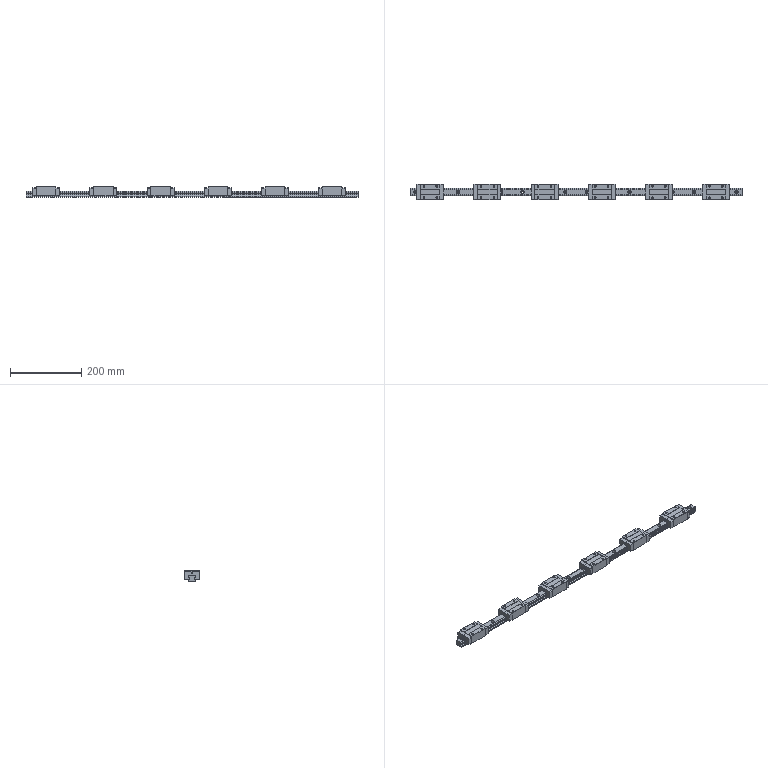Part | SolidWorks | 7 solids | 644 faces | box 930 x 44 x 30 mm | volume 645154 mm3 | plane 352 | cylinder 196 | cone 96 | commonest cylinder face diameters 4.3 x48 7.4 x48 9.5 x32 5 x24 6 x20 5.5 x12